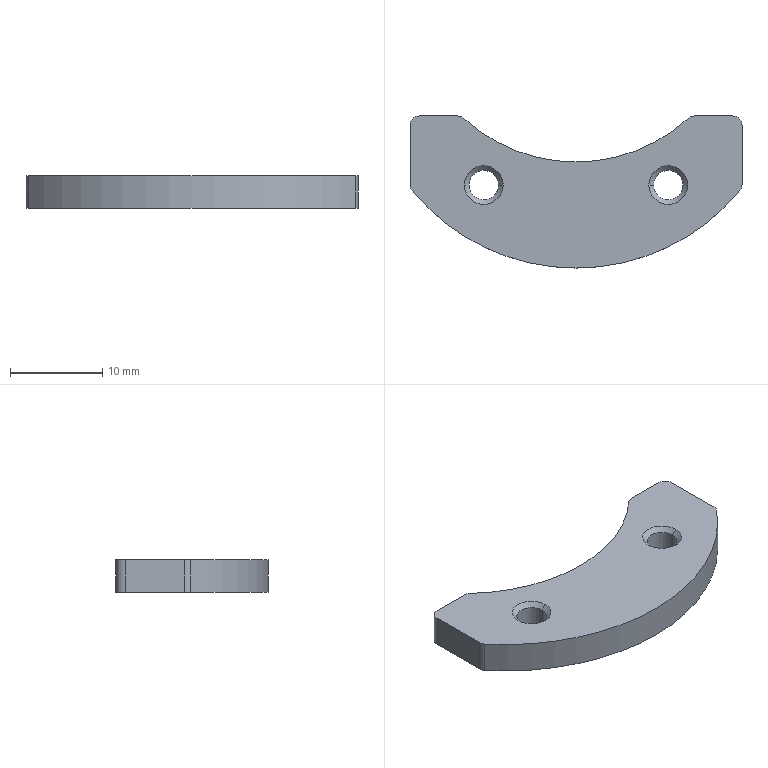Part | SolidWorks | features BaseBody 1 | 1 solid | 26 faces | box 36 x 16.5 x 3.5 mm | volume 1384 mm3 | cylinder 12 | cone 8 | plane 6 | commonest cylinder face diameters 2 x6 3.2 x4 36 x1 46 x1
STEP:
#1=CARTESIAN_POINT('',(-11.6,-20.5,3.));
#2=VERTEX_POINT('',#1);
#3=CARTESIAN_POINT('',(-8.4,-20.5,3.));
#4=VERTEX_POINT('',#3);
#5=CARTESIAN_POINT('',(-10.,-20.5,3.));
#6=DIRECTION('',(0.,0.,1.));
#7=DIRECTION('',(-1.,0.,0.));
#8=AXIS2_PLACEMENT_3D('',#5,#6,#7);
#9=CIRCLE('',#8,1.6);
#10=EDGE_CURVE('',#2,#4,#9,.T.);
#11=ORIENTED_EDGE('',*,*,#10,.F.);
#12=CARTESIAN_POINT('',(-12.1,-20.5,3.5));
#13=VERTEX_POINT('',#12);
#14=CARTESIAN_POINT('',(-11.6,-20.5,3.));
#15=DIRECTION('',(-0.7071,0.,0.7071));
#16=VECTOR('',#15,1000.);
#17=LINE('',#14,#16);
#18=EDGE_CURVE('',#2,#13,#17,.T.);
#19=ORIENTED_EDGE('',*,*,#18,.T.);
#20=CARTESIAN_POINT('',(-7.9,-20.5,3.5));
#21=VERTEX_POINT('',#20);
#22=CARTESIAN_POINT('',(-10.,-20.5,3.5));
#23=DIRECTION('',(0.,0.,-1.));
#24=DIRECTION('',(-1.,0.,0.));
#25=AXIS2_PLACEMENT_3D('',#22,#23,#24);
#26=CIRCLE('',#25,2.1);
#27=EDGE_CURVE('',#21,#13,#26,.T.);
#28=ORIENTED_EDGE('',*,*,#27,.F.);
#29=CARTESIAN_POINT('',(-8.4,-20.5,3.));
#30=DIRECTION('',(0.7071,0.,0.7071));
#31=VECTOR('',#30,1000.);
#32=LINE('',#29,#31);
#33=EDGE_CURVE('',#4,#21,#32,.T.);
#34=ORIENTED_EDGE('',*,*,#33,.F.);
#35=EDGE_LOOP('',(#11,#19,#28,#34));
#36=FACE_OUTER_BOUND('',#35,.T.);
#37=CARTESIAN_POINT('',(-10.,-20.5,3.));
#38=DIRECTION('',(0.,0.,1.));
#39=DIRECTION('',(1.,0.,0.));
#40=AXIS2_PLACEMENT_3D('',#37,#38,#39);
#41=CONICAL_SURFACE('',#40,1.6,0.7854);
#42=ADVANCED_FACE('',(#36),#41,.F.);
#43=CARTESIAN_POINT('',(-8.4,-20.5,0.5));
#44=VERTEX_POINT('',#43);
#45=CARTESIAN_POINT('',(-11.6,-20.5,0.5));
#46=VERTEX_POINT('',#45);
#47=CARTESIAN_POINT('',(-10.,-20.5,0.5));
#48=DIRECTION('',(0.,0.,-1.));
#49=DIRECTION('',(-1.,0.,0.));
#50=AXIS2_PLACEMENT_3D('',#47,#48,#49);
#51=CIRCLE('',#50,1.6);
#52=EDGE_CURVE('',#44,#46,#51,.T.);
#53=ORIENTED_EDGE('',*,*,#52,.F.);
#54=CARTESIAN_POINT('',(-7.9,-20.5,0.));
#55=VERTEX_POINT('',#54);
#56=CARTESIAN_POINT('',(-7.9,-20.5,0.));
#57=DIRECTION('',(0.7071,0.,-0.7071));
#58=VECTOR('',#57,1000.);
#59=LINE('',#56,#58);
#60=EDGE_CURVE('',#44,#55,#59,.T.);
#61=ORIENTED_EDGE('',*,*,#60,.T.);
#62=CARTESIAN_POINT('',(-12.1,-20.5,0.));
#63=VERTEX_POINT('',#62);
#64=CARTESIAN_POINT('',(-10.,-20.5,0.));
#65=DIRECTION('',(0.,0.,1.));
#66=DIRECTION('',(-1.,0.,0.));
#67=AXIS2_PLACEMENT_3D('',#64,#65,#66);
#68=CIRCLE('',#67,2.1);
#69=EDGE_CURVE('',#63,#55,#68,.T.);
#70=ORIENTED_EDGE('',*,*,#69,.F.);
#71=CARTESIAN_POINT('',(-12.1,-20.5,0.));
#72=DIRECTION('',(-0.7071,0.,-0.7071));
#73=VECTOR('',#72,1000.);
#74=LINE('',#71,#73);
#75=EDGE_CURVE('',#46,#63,#74,.T.);
#76=ORIENTED_EDGE('',*,*,#75,.F.);
#77=EDGE_LOOP('',(#53,#61,#70,#76));
#78=FACE_OUTER_BOUND('',#77,.T.);
#79=CARTESIAN_POINT('',(-10.,-20.5,0.));
#80=DIRECTION('',(0.,0.,-1.));
#81=DIRECTION('',(-1.,0.,0.));
#82=AXIS2_PLACEMENT_3D('',#79,#80,#81);
#83=CONICAL_SURFACE('',#82,2.1,0.7854);
#84=ADVANCED_FACE('',(#78),#83,.F.);
#85=CARTESIAN_POINT('',(8.4,-20.5,3.));
#86=VERTEX_POINT('',#85);
#87=CARTESIAN_POINT('',(11.6,-20.5,3.));
#88=VERTEX_POINT('',#87);
#89=CARTESIAN_POINT('',(10.,-20.5,3.));
#90=DIRECTION('',(0.,0.,1.));
#91=DIRECTION('',(-1.,0.,0.));
#92=AXIS2_PLACEMENT_3D('',#89,#90,#91);
#93=CIRCLE('',#92,1.6);
#94=EDGE_CURVE('',#86,#88,#93,.T.);
#95=ORIENTED_EDGE('',*,*,#94,.F.);
#96=CARTESIAN_POINT('',(7.9,-20.5,3.5));
#97=VERTEX_POINT('',#96);
#98=CARTESIAN_POINT('',(8.4,-20.5,3.));
#99=DIRECTION('',(-0.7071,0.,0.7071));
#100=VECTOR('',#99,1000.);
#101=LINE('',#98,#100);
#102=EDGE_CURVE('',#86,#97,#101,.T.);
#103=ORIENTED_EDGE('',*,*,#102,.T.);
#104=CARTESIAN_POINT('',(12.1,-20.5,3.5));
#105=VERTEX_POINT('',#104);
#106=CARTESIAN_POINT('',(10.,-20.5,3.5));
#107=DIRECTION('',(0.,0.,-1.));
#108=DIRECTION('',(-1.,0.,0.));
#109=AXIS2_PLACEMENT_3D('',#106,#107,#108);
#110=CIRCLE('',#109,2.1);
#111=EDGE_CURVE('',#105,#97,#110,.T.);
#112=ORIENTED_EDGE('',*,*,#111,.F.);
#113=CARTESIAN_POINT('',(11.6,-20.5,3.));
#114=DIRECTION('',(0.7071,0.,0.7071));
#115=VECTOR('',#114,1000.);
#116=LINE('',#113,#115);
#117=EDGE_CURVE('',#88,#105,#116,.T.);
#118=ORIENTED_EDGE('',*,*,#117,.F.);
#119=EDGE_LOOP('',(#95,#103,#112,#118));
#120=FACE_OUTER_BOUND('',#119,.T.);
#121=CARTESIAN_POINT('',(10.,-20.5,3.));
#122=DIRECTION('',(0.,0.,1.));
#123=DIRECTION('',(1.,0.,0.));
#124=AXIS2_PLACEMENT_3D('',#121,#122,#123);
#125=CONICAL_SURFACE('',#124,1.6,0.7854);
#126=ADVANCED_FACE('',(#120),#125,.F.);
#127=CARTESIAN_POINT('',(11.6,-20.5,0.5));
#128=VERTEX_POINT('',#127);
#129=CARTESIAN_POINT('',(8.4,-20.5,0.5));
#130=VERTEX_POINT('',#129);
#131=CARTESIAN_POINT('',(10.,-20.5,0.5));
#132=DIRECTION('',(0.,0.,-1.));
#133=DIRECTION('',(-1.,0.,0.));
#134=AXIS2_PLACEMENT_3D('',#131,#132,#133);
#135=CIRCLE('',#134,1.6);
#136=EDGE_CURVE('',#128,#130,#135,.T.);
#137=ORIENTED_EDGE('',*,*,#136,.F.);
#138=CARTESIAN_POINT('',(12.1,-20.5,0.));
#139=VERTEX_POINT('',#138);
#140=CARTESIAN_POINT('',(12.1,-20.5,0.));
#141=DIRECTION('',(0.7071,0.,-0.7071));
#142=VECTOR('',#141,1000.);
#143=LINE('',#140,#142);
#144=EDGE_CURVE('',#128,#139,#143,.T.);
#145=ORIENTED_EDGE('',*,*,#144,.T.);
#146=CARTESIAN_POINT('',(7.9,-20.5,0.));
#147=VERTEX_POINT('',#146);
#148=CARTESIAN_POINT('',(10.,-20.5,0.));
#149=DIRECTION('',(0.,0.,1.));
#150=DIRECTION('',(-1.,0.,0.));
#151=AXIS2_PLACEMENT_3D('',#148,#149,#150);
#152=CIRCLE('',#151,2.1);
#153=EDGE_CURVE('',#147,#139,#152,.T.);
#154=ORIENTED_EDGE('',*,*,#153,.F.);
#155=CARTESIAN_POINT('',(7.9,-20.5,0.));
#156=DIRECTION('',(-0.7071,0.,-0.7071));
#157=VECTOR('',#156,1000.);
#158=LINE('',#155,#157);
#159=EDGE_CURVE('',#130,#147,#158,.T.);
#160=ORIENTED_EDGE('',*,*,#159,.F.);
#161=EDGE_LOOP('',(#137,#145,#154,#160));
#162=FACE_OUTER_BOUND('',#161,.T.);
#163=CARTESIAN_POINT('',(10.,-20.5,0.));
#164=DIRECTION('',(0.,0.,-1.));
#165=DIRECTION('',(-1.,0.,0.));
#166=AXIS2_PLACEMENT_3D('',#163,#164,#165);
#167=CONICAL_SURFACE('',#166,2.1,0.7854);
#168=ADVANCED_FACE('',(#162),#167,.F.);
#169=ORIENTED_EDGE('',*,*,#94,.T.);
#170=CARTESIAN_POINT('',(11.6,-20.5,3.5));
#171=DIRECTION('',(0.,0.,-1.));
#172=VECTOR('',#171,1000.);
#173=LINE('',#170,#172);
#174=EDGE_CURVE('',#88,#128,#173,.T.);
#175=ORIENTED_EDGE('',*,*,#174,.T.);
#176=ORIENTED_EDGE('',*,*,#136,.T.);
#177=CARTESIAN_POINT('',(8.4,-20.5,3.5));
#178=DIRECTION('',(0.,0.,-1.));
#179=VECTOR('',#178,1000.);
#180=LINE('',#177,#179);
#181=EDGE_CURVE('',#86,#130,#180,.T.);
#182=ORIENTED_EDGE('',*,*,#181,.F.);
#183=EDGE_LOOP('',(#169,#175,#176,#182));
#184=FACE_OUTER_BOUND('',#183,.T.);
#185=CARTESIAN_POINT('',(10.,-20.5,3.5));
#186=DIRECTION('',(0.,0.,-1.));
#187=DIRECTION('',(-1.,0.,0.));
#188=AXIS2_PLACEMENT_3D('',#185,#186,#187);
#189=CYLINDRICAL_SURFACE('',#188,1.6);
#190=ADVANCED_FACE('',(#184),#189,.F.);
#191=ORIENTED_EDGE('',*,*,#10,.T.);
#192=CARTESIAN_POINT('',(-8.4,-20.5,3.5));
#193=DIRECTION('',(0.,0.,-1.));
#194=VECTOR('',#193,1000.);
#195=LINE('',#192,#194);
#196=EDGE_CURVE('',#4,#44,#195,.T.);
#197=ORIENTED_EDGE('',*,*,#196,.T.);
#198=ORIENTED_EDGE('',*,*,#52,.T.);
#199=CARTESIAN_POINT('',(-11.6,-20.5,3.5));
#200=DIRECTION('',(0.,0.,-1.));
#201=VECTOR('',#200,1000.);
#202=LINE('',#199,#201);
#203=EDGE_CURVE('',#2,#46,#202,.T.);
#204=ORIENTED_EDGE('',*,*,#203,.F.);
#205=EDGE_LOOP('',(#191,#197,#198,#204));
#206=FACE_OUTER_BOUND('',#205,.T.);
#207=CARTESIAN_POINT('',(-10.,-20.5,3.5));
#208=DIRECTION('',(0.,0.,-1.));
#209=DIRECTION('',(-1.,0.,0.));
#210=AXIS2_PLACEMENT_3D('',#207,#208,#209);
#211=CYLINDRICAL_SURFACE('',#210,1.6);
#212=ADVANCED_FACE('',(#206),#211,.F.);
#213=ORIENTED_EDGE('',*,*,#111,.T.);
#214=CARTESIAN_POINT('',(10.,-20.5,3.5));
#215=DIRECTION('',(0.,0.,-1.));
#216=DIRECTION('',(-1.,0.,0.));
#217=AXIS2_PLACEMENT_3D('',#214,#215,#216);
#218=CIRCLE('',#217,2.1);
#219=EDGE_CURVE('',#97,#105,#218,.T.);
#220=ORIENTED_EDGE('',*,*,#219,.T.);
#221=EDGE_LOOP('',(#213,#220));
#222=FACE_BOUND('',#221,.T.);
#223=ORIENTED_EDGE('',*,*,#27,.T.);
#224=CARTESIAN_POINT('',(-10.,-20.5,3.5));
#225=DIRECTION('',(0.,0.,-1.));
#226=DIRECTION('',(-1.,0.,0.));
#227=AXIS2_PLACEMENT_3D('',#224,#225,#226);
#228=CIRCLE('',#227,2.1);
#229=EDGE_CURVE('',#13,#21,#228,.T.);
#230=ORIENTED_EDGE('',*,*,#229,.T.);
#231=EDGE_LOOP('',(#223,#230));
#232=FACE_BOUND('',#231,.T.);
#233=CARTESIAN_POINT('',(-18.,-20.464,3.5));
#234=VERTEX_POINT('',#233);
#235=CARTESIAN_POINT('',(-17.773,-21.099,3.5));
#236=VERTEX_POINT('',#235);
#237=CARTESIAN_POINT('',(-17.,-20.464,3.5));
#238=DIRECTION('',(0.,0.,1.));
#239=DIRECTION('',(-1.,0.,0.));
#240=AXIS2_PLACEMENT_3D('',#237,#238,#239);
#241=CIRCLE('',#240,1.);
#242=EDGE_CURVE('',#234,#236,#241,.T.);
#243=ORIENTED_EDGE('',*,*,#242,.T.);
#244=CARTESIAN_POINT('',(17.773,-21.099,3.5));
#245=VERTEX_POINT('',#244);
#246=CARTESIAN_POINT('',(0.,-6.5,3.5));
#247=DIRECTION('',(0.,0.,1.));
#248=DIRECTION('',(1.,0.,0.));
#249=AXIS2_PLACEMENT_3D('',#246,#247,#248);
#250=CIRCLE('',#249,23.);
#251=EDGE_CURVE('',#236,#245,#250,.T.);
#252=ORIENTED_EDGE('',*,*,#251,.T.);
#253=CARTESIAN_POINT('',(18.,-20.464,3.5));
#254=VERTEX_POINT('',#253);
#255=CARTESIAN_POINT('',(17.,-20.464,3.5));
#256=DIRECTION('',(0.,0.,1.));
#257=DIRECTION('',(-1.,0.,0.));
#258=AXIS2_PLACEMENT_3D('',#255,#256,#257);
#259=CIRCLE('',#258,1.);
#260=EDGE_CURVE('',#245,#254,#259,.T.);
#261=ORIENTED_EDGE('',*,*,#260,.T.);
#262=CARTESIAN_POINT('',(18.,-14.,3.5));
#263=VERTEX_POINT('',#262);
#264=CARTESIAN_POINT('',(18.,-20.464,3.5));
#265=DIRECTION('',(0.,1.,0.));
#266=VECTOR('',#265,1000.);
#267=LINE('',#264,#266);
#268=EDGE_CURVE('',#254,#263,#267,.T.);
#269=ORIENTED_EDGE('',*,*,#268,.T.);
#270=CARTESIAN_POINT('',(17.,-13.,3.5));
#271=VERTEX_POINT('',#270);
#272=CARTESIAN_POINT('',(17.,-14.,3.5));
#273=DIRECTION('',(0.,0.,1.));
#274=DIRECTION('',(1.,0.,0.));
#275=AXIS2_PLACEMENT_3D('',#272,#273,#274);
#276=CIRCLE('',#275,1.);
#277=EDGE_CURVE('',#263,#271,#276,.T.);
#278=ORIENTED_EDGE('',*,*,#277,.T.);
#279=CARTESIAN_POINT('',(12.845,-13.,3.5));
#280=VERTEX_POINT('',#279);
#281=CARTESIAN_POINT('',(12.845,-13.,3.5));
#282=DIRECTION('',(-1.,0.,0.));
#283=VECTOR('',#282,1000.);
#284=LINE('',#281,#283);
#285=EDGE_CURVE('',#271,#280,#284,.T.);
#286=ORIENTED_EDGE('',*,*,#285,.T.);
#287=CARTESIAN_POINT('',(12.169,-13.263,3.5));
#288=VERTEX_POINT('',#287);
#289=CARTESIAN_POINT('',(12.845,-14.,3.5));
#290=DIRECTION('',(0.,0.,1.));
#291=DIRECTION('',(1.,0.,0.));
#292=AXIS2_PLACEMENT_3D('',#289,#290,#291);
#293=CIRCLE('',#292,1.);
#294=EDGE_CURVE('',#280,#288,#293,.T.);
#295=ORIENTED_EDGE('',*,*,#294,.T.);
#296=CARTESIAN_POINT('',(-12.169,-13.263,3.5));
#297=VERTEX_POINT('',#296);
#298=CARTESIAN_POINT('',(0.,0.,3.5));
#299=DIRECTION('',(0.,0.,-1.));
#300=DIRECTION('',(1.,0.,0.));
#301=AXIS2_PLACEMENT_3D('',#298,#299,#300);
#302=CIRCLE('',#301,18.);
#303=EDGE_CURVE('',#288,#297,#302,.T.);
#304=ORIENTED_EDGE('',*,*,#303,.T.);
#305=CARTESIAN_POINT('',(-12.845,-13.,3.5));
#306=VERTEX_POINT('',#305);
#307=CARTESIAN_POINT('',(-12.845,-14.,3.5));
#308=DIRECTION('',(0.,0.,1.));
#309=DIRECTION('',(1.,0.,0.));
#310=AXIS2_PLACEMENT_3D('',#307,#308,#309);
#311=CIRCLE('',#310,1.);
#312=EDGE_CURVE('',#297,#306,#311,.T.);
#313=ORIENTED_EDGE('',*,*,#312,.T.);
#314=CARTESIAN_POINT('',(-17.,-13.,3.5));
#315=VERTEX_POINT('',#314);
#316=CARTESIAN_POINT('',(-17.,-13.,3.5));
#317=DIRECTION('',(-1.,0.,0.));
#318=VECTOR('',#317,1000.);
#319=LINE('',#316,#318);
#320=EDGE_CURVE('',#306,#315,#319,.T.);
#321=ORIENTED_EDGE('',*,*,#320,.T.);
#322=CARTESIAN_POINT('',(-18.,-14.,3.5));
#323=VERTEX_POINT('',#322);
#324=CARTESIAN_POINT('',(-17.,-14.,3.5));
#325=DIRECTION('',(0.,0.,1.));
#326=DIRECTION('',(1.,0.,0.));
#327=AXIS2_PLACEMENT_3D('',#324,#325,#326);
#328=CIRCLE('',#327,1.);
#329=EDGE_CURVE('',#315,#323,#328,.T.);
#330=ORIENTED_EDGE('',*,*,#329,.T.);
#331=CARTESIAN_POINT('',(-18.,-20.464,3.5));
#332=DIRECTION('',(0.,-1.,0.));
#333=VECTOR('',#332,1000.);
#334=LINE('',#331,#333);
#335=EDGE_CURVE('',#323,#234,#334,.T.);
#336=ORIENTED_EDGE('',*,*,#335,.T.);
#337=EDGE_LOOP('',(#243,#252,#261,#269,#278,#286,#295,#304,#313,#321,#330,#336));
#338=FACE_OUTER_BOUND('',#337,.T.);
#339=CARTESIAN_POINT('',(-17.,-20.464,3.5));
#340=DIRECTION('',(0.,0.,-1.));
#341=DIRECTION('',(-1.,0.,0.));
#342=AXIS2_PLACEMENT_3D('',#339,#340,#341);
#343=PLANE('',#342);
#344=ADVANCED_FACE('',(#222,#232,#338),#343,.F.);
#345=ORIENTED_EDGE('',*,*,#153,.T.);
#346=CARTESIAN_POINT('',(10.,-20.5,0.));
#347=DIRECTION('',(0.,0.,1.));
#348=DIRECTION('',(-1.,0.,0.));
#349=AXIS2_PLACEMENT_3D('',#346,#347,#348);
#350=CIRCLE('',#349,2.1);
#351=EDGE_CURVE('',#139,#147,#350,.T.);
#352=ORIENTED_EDGE('',*,*,#351,.T.);
#353=EDGE_LOOP('',(#345,#352));
#354=FACE_BOUND('',#353,.T.);
#355=ORIENTED_EDGE('',*,*,#69,.T.);
#356=CARTESIAN_POINT('',(-10.,-20.5,0.));
#357=DIRECTION('',(0.,0.,1.));
#358=DIRECTION('',(-1.,0.,0.));
#359=AXIS2_PLACEMENT_3D('',#356,#357,#358);
#360=CIRCLE('',#359,2.1);
#361=EDGE_CURVE('',#55,#63,#360,.T.);
#362=ORIENTED_EDGE('',*,*,#361,.T.);
#363=EDGE_LOOP('',(#355,#362));
#364=FACE_BOUND('',#363,.T.);
#365=CARTESIAN_POINT('',(-18.,-20.464,0.));
#366=VERTEX_POINT('',#365);
#367=CARTESIAN_POINT('',(-17.773,-21.099,0.));
#368=VERTEX_POINT('',#367);
#369=CARTESIAN_POINT('',(-17.,-20.464,0.));
#370=DIRECTION('',(0.,0.,1.));
#371=DIRECTION('',(-1.,0.,0.));
#372=AXIS2_PLACEMENT_3D('',#369,#370,#371);
#373=CIRCLE('',#372,1.);
#374=EDGE_CURVE('',#366,#368,#373,.T.);
#375=ORIENTED_EDGE('',*,*,#374,.F.);
#376=CARTESIAN_POINT('',(-18.,-14.,0.));
#377=VERTEX_POINT('',#376);
#378=CARTESIAN_POINT('',(-18.,-20.464,0.));
#379=DIRECTION('',(0.,-1.,0.));
#380=VECTOR('',#379,1000.);
#381=LINE('',#378,#380);
#382=EDGE_CURVE('',#377,#366,#381,.T.);
#383=ORIENTED_EDGE('',*,*,#382,.F.);
#384=CARTESIAN_POINT('',(-17.,-13.,0.));
#385=VERTEX_POINT('',#384);
#386=CARTESIAN_POINT('',(-17.,-14.,0.));
#387=DIRECTION('',(0.,0.,1.));
#388=DIRECTION('',(1.,0.,0.));
#389=AXIS2_PLACEMENT_3D('',#386,#387,#388);
#390=CIRCLE('',#389,1.);
#391=EDGE_CURVE('',#385,#377,#390,.T.);
#392=ORIENTED_EDGE('',*,*,#391,.F.);
#393=CARTESIAN_POINT('',(-12.845,-13.,0.));
#394=VERTEX_POINT('',#393);
#395=CARTESIAN_POINT('',(-17.,-13.,0.));
#396=DIRECTION('',(-1.,0.,0.));
#397=VECTOR('',#396,1000.);
#398=LINE('',#395,#397);
#399=EDGE_CURVE('',#394,#385,#398,.T.);
#400=ORIENTED_EDGE('',*,*,#399,.F.);
#401=CARTESIAN_POINT('',(-12.169,-13.263,0.));
#402=VERTEX_POINT('',#401);
#403=CARTESIAN_POINT('',(-12.845,-14.,0.));
#404=DIRECTION('',(0.,0.,1.));
#405=DIRECTION('',(1.,0.,0.));
#406=AXIS2_PLACEMENT_3D('',#403,#404,#405);
#407=CIRCLE('',#406,1.);
#408=EDGE_CURVE('',#402,#394,#407,.T.);
#409=ORIENTED_EDGE('',*,*,#408,.F.);
#410=CARTESIAN_POINT('',(12.169,-13.263,0.));
#411=VERTEX_POINT('',#410);
#412=CARTESIAN_POINT('',(0.,0.,0.));
#413=DIRECTION('',(0.,0.,-1.));
#414=DIRECTION('',(1.,0.,0.));
#415=AXIS2_PLACEMENT_3D('',#412,#413,#414);
#416=CIRCLE('',#415,18.);
#417=EDGE_CURVE('',#411,#402,#416,.T.);
#418=ORIENTED_EDGE('',*,*,#417,.F.);
#419=CARTESIAN_POINT('',(12.845,-13.,0.));
#420=VERTEX_POINT('',#419);
#421=CARTESIAN_POINT('',(12.845,-14.,0.));
#422=DIRECTION('',(0.,0.,1.));
#423=DIRECTION('',(1.,0.,0.));
#424=AXIS2_PLACEMENT_3D('',#421,#422,#423);
#425=CIRCLE('',#424,1.);
#426=EDGE_CURVE('',#420,#411,#425,.T.);
#427=ORIENTED_EDGE('',*,*,#426,.F.);
#428=CARTESIAN_POINT('',(17.,-13.,0.));
#429=VERTEX_POINT('',#428);
#430=CARTESIAN_POINT('',(12.845,-13.,0.));
#431=DIRECTION('',(-1.,0.,0.));
#432=VECTOR('',#431,1000.);
#433=LINE('',#430,#432);
#434=EDGE_CURVE('',#429,#420,#433,.T.);
#435=ORIENTED_EDGE('',*,*,#434,.F.);
#436=CARTESIAN_POINT('',(18.,-14.,0.));
#437=VERTEX_POINT('',#436);
#438=CARTESIAN_POINT('',(17.,-14.,0.));
#439=DIRECTION('',(0.,0.,1.));
#440=DIRECTION('',(1.,0.,0.));
#441=AXIS2_PLACEMENT_3D('',#438,#439,#440);
#442=CIRCLE('',#441,1.);
#443=EDGE_CURVE('',#437,#429,#442,.T.);
#444=ORIENTED_EDGE('',*,*,#443,.F.);
#445=CARTESIAN_POINT('',(18.,-20.464,0.));
#446=VERTEX_POINT('',#445);
#447=CARTESIAN_POINT('',(18.,-20.464,0.));
#448=DIRECTION('',(0.,1.,0.));
#449=VECTOR('',#448,1000.);
#450=LINE('',#447,#449);
#451=EDGE_CURVE('',#446,#437,#450,.T.);
#452=ORIENTED_EDGE('',*,*,#451,.F.);
#453=CARTESIAN_POINT('',(17.773,-21.099,0.));
#454=VERTEX_POINT('',#453);
#455=CARTESIAN_POINT('',(17.,-20.464,0.));
#456=DIRECTION('',(0.,0.,1.));
#457=DIRECTION('',(-1.,0.,0.));
#458=AXIS2_PLACEMENT_3D('',#455,#456,#457);
#459=CIRCLE('',#458,1.);
#460=EDGE_CURVE('',#454,#446,#459,.T.);
#461=ORIENTED_EDGE('',*,*,#460,.F.);
#462=CARTESIAN_POINT('',(0.,-6.5,0.));
#463=DIRECTION('',(0.,0.,1.));
#464=DIRECTION('',(1.,0.,0.));
#465=AXIS2_PLACEMENT_3D('',#462,#463,#464);
#466=CIRCLE('',#465,23.);
#467=EDGE_CURVE('',#368,#454,#466,.T.);
#468=ORIENTED_EDGE('',*,*,#467,.F.);
#469=EDGE_LOOP('',(#375,#383,#392,#400,#409,#418,#427,#435,#444,#452,#461,#468));
#470=FACE_OUTER_BOUND('',#469,.T.);
#471=CARTESIAN_POINT('',(-17.,-20.464,0.));
#472=DIRECTION('',(0.,0.,-1.));
#473=DIRECTION('',(-1.,0.,0.));
#474=AXIS2_PLACEMENT_3D('',#471,#472,#473);
#475=PLANE('',#474);
#476=ADVANCED_FACE('',(#354,#364,#470),#475,.T.);
#477=ORIENTED_EDGE('',*,*,#374,.T.);
#478=CARTESIAN_POINT('',(-17.773,-21.099,3.5));
#479=DIRECTION('',(0.,0.,-1.));
#480=VECTOR('',#479,1000.);
#481=LINE('',#478,#480);
#482=EDGE_CURVE('',#236,#368,#481,.T.);
#483=ORIENTED_EDGE('',*,*,#482,.F.);
#484=ORIENTED_EDGE('',*,*,#242,.F.);
#485=CARTESIAN_POINT('',(-18.,-20.464,3.5));
#486=DIRECTION('',(0.,0.,-1.));
#487=VECTOR('',#486,1000.);
#488=LINE('',#485,#487);
#489=EDGE_CURVE('',#234,#366,#488,.T.);
#490=ORIENTED_EDGE('',*,*,#489,.T.);
#491=EDGE_LOOP('',(#477,#483,#484,#490));
#492=FACE_OUTER_BOUND('',#491,.T.);
#493=CARTESIAN_POINT('',(-17.,-20.464,3.5));
#494=DIRECTION('',(0.,0.,-1.));
#495=DIRECTION('',(-1.,0.,0.));
#496=AXIS2_PLACEMENT_3D('',#493,#494,#495);
#497=CYLINDRICAL_SURFACE('',#496,1.);
#498=ADVANCED_FACE('',(#492),#497,.T.);
#499=ORIENTED_EDGE('',*,*,#467,.T.);
#500=CARTESIAN_POINT('',(17.773,-21.099,3.5));
#501=DIRECTION('',(0.,0.,-1.));
#502=VECTOR('',#501,1000.);
#503=LINE('',#500,#502);
#504=EDGE_CURVE('',#245,#454,#503,.T.);
#505=ORIENTED_EDGE('',*,*,#504,.F.);
#506=ORIENTED_EDGE('',*,*,#251,.F.);
#507=ORIENTED_EDGE('',*,*,#482,.T.);
#508=EDGE_LOOP('',(#499,#505,#506,#507));
#509=FACE_OUTER_BOUND('',#508,.T.);
#510=CARTESIAN_POINT('',(0.,-6.5,3.5));
#511=DIRECTION('',(0.,0.,-1.));
#512=DIRECTION('',(-1.,0.,0.));
#513=AXIS2_PLACEMENT_3D('',#510,#511,#512);
#514=CYLINDRICAL_SURFACE('',#513,23.);
#515=ADVANCED_FACE('',(#509),#514,.T.);
#516=ORIENTED_EDGE('',*,*,#460,.T.);
#517=CARTESIAN_POINT('',(18.,-20.464,3.5));
#518=DIRECTION('',(0.,0.,-1.));
#519=VECTOR('',#518,1000.);
#520=LINE('',#517,#519);
#521=EDGE_CURVE('',#254,#446,#520,.T.);
#522=ORIENTED_EDGE('',*,*,#521,.F.);
#523=ORIENTED_EDGE('',*,*,#260,.F.);
#524=ORIENTED_EDGE('',*,*,#504,.T.);
#525=EDGE_LOOP('',(#516,#522,#523,#524));
#526=FACE_OUTER_BOUND('',#525,.T.);
#527=CARTESIAN_POINT('',(17.,-20.464,3.5));
#528=DIRECTION('',(0.,0.,-1.));
#529=DIRECTION('',(-1.,0.,0.));
#530=AXIS2_PLACEMENT_3D('',#527,#528,#529);
#531=CYLINDRICAL_SURFACE('',#530,1.);
#532=ADVANCED_FACE('',(#526),#531,.T.);
#533=ORIENTED_EDGE('',*,*,#451,.T.);
#534=CARTESIAN_POINT('',(18.,-14.,3.5));
#535=DIRECTION('',(0.,0.,-1.));
#536=VECTOR('',#535,1000.);
#537=LINE('',#534,#536);
#538=EDGE_CURVE('',#263,#437,#537,.T.);
#539=ORIENTED_EDGE('',*,*,#538,.F.);
#540=ORIENTED_EDGE('',*,*,#268,.F.);
#541=ORIENTED_EDGE('',*,*,#521,.T.);
#542=EDGE_LOOP('',(#533,#539,#540,#541));
#543=FACE_OUTER_BOUND('',#542,.T.);
#544=CARTESIAN_POINT('',(18.,-20.464,3.5));
#545=DIRECTION('',(-1.,0.,0.));
#546=DIRECTION('',(0.,0.,1.));
#547=AXIS2_PLACEMENT_3D('',#544,#545,#546);
#548=PLANE('',#547);
#549=ADVANCED_FACE('',(#543),#548,.F.);
#550=ORIENTED_EDGE('',*,*,#443,.T.);
#551=CARTESIAN_POINT('',(17.,-13.,3.5));
#552=DIRECTION('',(0.,0.,-1.));
#553=VECTOR('',#552,1000.);
#554=LINE('',#551,#553);
#555=EDGE_CURVE('',#271,#429,#554,.T.);
#556=ORIENTED_EDGE('',*,*,#555,.F.);
#557=ORIENTED_EDGE('',*,*,#277,.F.);
#558=ORIENTED_EDGE('',*,*,#538,.T.);
#559=EDGE_LOOP('',(#550,#556,#557,#558));
#560=FACE_OUTER_BOUND('',#559,.T.);
#561=CARTESIAN_POINT('',(17.,-14.,3.5));
#562=DIRECTION('',(0.,0.,-1.));
#563=DIRECTION('',(-1.,0.,0.));
#564=AXIS2_PLACEMENT_3D('',#561,#562,#563);
#565=CYLINDRICAL_SURFACE('',#564,1.);
#566=ADVANCED_FACE('',(#560),#565,.T.);
#567=ORIENTED_EDGE('',*,*,#434,.T.);
#568=CARTESIAN_POINT('',(12.845,-13.,3.5));
#569=DIRECTION('',(0.,0.,-1.));
#570=VECTOR('',#569,1000.);
#571=LINE('',#568,#570);
#572=EDGE_CURVE('',#280,#420,#571,.T.);
#573=ORIENTED_EDGE('',*,*,#572,.F.);
#574=ORIENTED_EDGE('',*,*,#285,.F.);
#575=ORIENTED_EDGE('',*,*,#555,.T.);
#576=EDGE_LOOP('',(#567,#573,#574,#575));
#577=FACE_OUTER_BOUND('',#576,.T.);
#578=CARTESIAN_POINT('',(12.845,-13.,3.5));
#579=DIRECTION('',(0.,-1.,0.));
#580=DIRECTION('',(0.,0.,-1.));
#581=AXIS2_PLACEMENT_3D('',#578,#579,#580);
#582=PLANE('',#581);
#583=ADVANCED_FACE('',(#577),#582,.F.);
#584=ORIENTED_EDGE('',*,*,#426,.T.);
#585=CARTESIAN_POINT('',(12.169,-13.263,3.5));
#586=DIRECTION('',(0.,0.,-1.));
#587=VECTOR('',#586,1000.);
#588=LINE('',#585,#587);
#589=EDGE_CURVE('',#288,#411,#588,.T.);
#590=ORIENTED_EDGE('',*,*,#589,.F.);
#591=ORIENTED_EDGE('',*,*,#294,.F.);
#592=ORIENTED_EDGE('',*,*,#572,.T.);
#593=EDGE_LOOP('',(#584,#590,#591,#592));
#594=FACE_OUTER_BOUND('',#593,.T.);
#595=CARTESIAN_POINT('',(12.845,-14.,3.5));
#596=DIRECTION('',(0.,0.,-1.));
#597=DIRECTION('',(-1.,0.,0.));
#598=AXIS2_PLACEMENT_3D('',#595,#596,#597);
#599=CYLINDRICAL_SURFACE('',#598,1.);
#600=ADVANCED_FACE('',(#594),#599,.T.);
#601=ORIENTED_EDGE('',*,*,#417,.T.);
#602=CARTESIAN_POINT('',(-12.169,-13.263,3.5));
#603=DIRECTION('',(0.,0.,-1.));
#604=VECTOR('',#603,1000.);
#605=LINE('',#602,#604);
#606=EDGE_CURVE('',#297,#402,#605,.T.);
#607=ORIENTED_EDGE('',*,*,#606,.F.);
#608=ORIENTED_EDGE('',*,*,#303,.F.);
#609=ORIENTED_EDGE('',*,*,#589,.T.);
#610=EDGE_LOOP('',(#601,#607,#608,#609));
#611=FACE_OUTER_BOUND('',#610,.T.);
#612=CARTESIAN_POINT('',(0.,0.,3.5));
#613=DIRECTION('',(0.,0.,-1.));
#614=DIRECTION('',(-1.,0.,0.));
#615=AXIS2_PLACEMENT_3D('',#612,#613,#614);
#616=CYLINDRICAL_SURFACE('',#615,18.);
#617=ADVANCED_FACE('',(#611),#616,.F.);
#618=ORIENTED_EDGE('',*,*,#408,.T.);
#619=CARTESIAN_POINT('',(-12.845,-13.,3.5));
#620=DIRECTION('',(0.,0.,-1.));
#621=VECTOR('',#620,1000.);
#622=LINE('',#619,#621);
#623=EDGE_CURVE('',#306,#394,#622,.T.);
#624=ORIENTED_EDGE('',*,*,#623,.F.);
#625=ORIENTED_EDGE('',*,*,#312,.F.);
#626=ORIENTED_EDGE('',*,*,#606,.T.);
#627=EDGE_LOOP('',(#618,#624,#625,#626));
#628=FACE_OUTER_BOUND('',#627,.T.);
#629=CARTESIAN_POINT('',(-12.845,-14.,3.5));
#630=DIRECTION('',(0.,0.,-1.));
#631=DIRECTION('',(-1.,0.,0.));
#632=AXIS2_PLACEMENT_3D('',#629,#630,#631);
#633=CYLINDRICAL_SURFACE('',#632,1.);
#634=ADVANCED_FACE('',(#628),#633,.T.);
#635=ORIENTED_EDGE('',*,*,#399,.T.);
#636=CARTESIAN_POINT('',(-17.,-13.,3.5));
#637=DIRECTION('',(0.,0.,-1.));
#638=VECTOR('',#637,1000.);
#639=LINE('',#636,#638);
#640=EDGE_CURVE('',#315,#385,#639,.T.);
#641=ORIENTED_EDGE('',*,*,#640,.F.);
#642=ORIENTED_EDGE('',*,*,#320,.F.);
#643=ORIENTED_EDGE('',*,*,#623,.T.);
#644=EDGE_LOOP('',(#635,#641,#642,#643));
#645=FACE_OUTER_BOUND('',#644,.T.);
#646=CARTESIAN_POINT('',(-17.,-13.,3.5));
#647=DIRECTION('',(0.,-1.,0.));
#648=DIRECTION('',(0.,0.,-1.));
#649=AXIS2_PLACEMENT_3D('',#646,#647,#648);
#650=PLANE('',#649);
#651=ADVANCED_FACE('',(#645),#650,.F.);
#652=ORIENTED_EDGE('',*,*,#391,.T.);
#653=CARTESIAN_POINT('',(-18.,-14.,3.5));
#654=DIRECTION('',(0.,0.,-1.));
#655=VECTOR('',#654,1000.);
#656=LINE('',#653,#655);
#657=EDGE_CURVE('',#323,#377,#656,.T.);
#658=ORIENTED_EDGE('',*,*,#657,.F.);
#659=ORIENTED_EDGE('',*,*,#329,.F.);
#660=ORIENTED_EDGE('',*,*,#640,.T.);
#661=EDGE_LOOP('',(#652,#658,#659,#660));
#662=FACE_OUTER_BOUND('',#661,.T.);
#663=CARTESIAN_POINT('',(-17.,-14.,3.5));
#664=DIRECTION('',(0.,0.,-1.));
#665=DIRECTION('',(-1.,0.,0.));
#666=AXIS2_PLACEMENT_3D('',#663,#664,#665);
#667=CYLINDRICAL_SURFACE('',#666,1.);
#668=ADVANCED_FACE('',(#662),#667,.T.);
#669=ORIENTED_EDGE('',*,*,#382,.T.);
#670=ORIENTED_EDGE('',*,*,#489,.F.);
#671=ORIENTED_EDGE('',*,*,#335,.F.);
#672=ORIENTED_EDGE('',*,*,#657,.T.);
#673=EDGE_LOOP('',(#669,#670,#671,#672));
#674=FACE_OUTER_BOUND('',#673,.T.);
#675=CARTESIAN_POINT('',(-18.,-20.464,3.5));
#676=DIRECTION('',(1.,0.,0.));
#677=DIRECTION('',(0.,0.,-1.));
#678=AXIS2_PLACEMENT_3D('',#675,#676,#677);
#679=PLANE('',#678);
#680=ADVANCED_FACE('',(#674),#679,.F.);
#681=ORIENTED_EDGE('',*,*,#196,.F.);
#682=CARTESIAN_POINT('',(-10.,-20.5,3.));
#683=DIRECTION('',(0.,0.,1.));
#684=DIRECTION('',(-1.,0.,0.));
#685=AXIS2_PLACEMENT_3D('',#682,#683,#684);
#686=CIRCLE('',#685,1.6);
#687=EDGE_CURVE('',#4,#2,#686,.T.);
#688=ORIENTED_EDGE('',*,*,#687,.T.);
#689=ORIENTED_EDGE('',*,*,#203,.T.);
#690=CARTESIAN_POINT('',(-10.,-20.5,0.5));
#691=DIRECTION('',(0.,0.,-1.));
#692=DIRECTION('',(-1.,0.,0.));
#693=AXIS2_PLACEMENT_3D('',#690,#691,#692);
#694=CIRCLE('',#693,1.6);
#695=EDGE_CURVE('',#46,#44,#694,.T.);
#696=ORIENTED_EDGE('',*,*,#695,.T.);
#697=EDGE_LOOP('',(#681,#688,#689,#696));
#698=FACE_OUTER_BOUND('',#697,.T.);
#699=CARTESIAN_POINT('',(-10.,-20.5,3.5));
#700=DIRECTION('',(0.,0.,-1.));
#701=DIRECTION('',(-1.,0.,0.));
#702=AXIS2_PLACEMENT_3D('',#699,#700,#701);
#703=CYLINDRICAL_SURFACE('',#702,1.6);
#704=ADVANCED_FACE('',(#698),#703,.F.);
#705=ORIENTED_EDGE('',*,*,#174,.F.);
#706=CARTESIAN_POINT('',(10.,-20.5,3.));
#707=DIRECTION('',(0.,0.,1.));
#708=DIRECTION('',(-1.,0.,0.));
#709=AXIS2_PLACEMENT_3D('',#706,#707,#708);
#710=CIRCLE('',#709,1.6);
#711=EDGE_CURVE('',#88,#86,#710,.T.);
#712=ORIENTED_EDGE('',*,*,#711,.T.);
#713=ORIENTED_EDGE('',*,*,#181,.T.);
#714=CARTESIAN_POINT('',(10.,-20.5,0.5));
#715=DIRECTION('',(0.,0.,-1.));
#716=DIRECTION('',(-1.,0.,0.));
#717=AXIS2_PLACEMENT_3D('',#714,#715,#716);
#718=CIRCLE('',#717,1.6);
#719=EDGE_CURVE('',#130,#128,#718,.T.);
#720=ORIENTED_EDGE('',*,*,#719,.T.);
#721=EDGE_LOOP('',(#705,#712,#713,#720));
#722=FACE_OUTER_BOUND('',#721,.T.);
#723=CARTESIAN_POINT('',(10.,-20.5,3.5));
#724=DIRECTION('',(0.,0.,-1.));
#725=DIRECTION('',(-1.,0.,0.));
#726=AXIS2_PLACEMENT_3D('',#723,#724,#725);
#727=CYLINDRICAL_SURFACE('',#726,1.6);
#728=ADVANCED_FACE('',(#722),#727,.F.);
#729=ORIENTED_EDGE('',*,*,#144,.F.);
#730=ORIENTED_EDGE('',*,*,#719,.F.);
#731=ORIENTED_EDGE('',*,*,#159,.T.);
#732=ORIENTED_EDGE('',*,*,#351,.F.);
#733=EDGE_LOOP('',(#729,#730,#731,#732));
#734=FACE_OUTER_BOUND('',#733,.T.);
#735=CARTESIAN_POINT('',(10.,-20.5,0.));
#736=DIRECTION('',(0.,0.,-1.));
#737=DIRECTION('',(-1.,0.,0.));
#738=AXIS2_PLACEMENT_3D('',#735,#736,#737);
#739=CONICAL_SURFACE('',#738,2.1,0.7854);
#740=ADVANCED_FACE('',(#734),#739,.F.);
#741=ORIENTED_EDGE('',*,*,#102,.F.);
#742=ORIENTED_EDGE('',*,*,#711,.F.);
#743=ORIENTED_EDGE('',*,*,#117,.T.);
#744=ORIENTED_EDGE('',*,*,#219,.F.);
#745=EDGE_LOOP('',(#741,#742,#743,#744));
#746=FACE_OUTER_BOUND('',#745,.T.);
#747=CARTESIAN_POINT('',(10.,-20.5,3.));
#748=DIRECTION('',(0.,0.,1.));
#749=DIRECTION('',(1.,0.,0.));
#750=AXIS2_PLACEMENT_3D('',#747,#748,#749);
#751=CONICAL_SURFACE('',#750,1.6,0.7854);
#752=ADVANCED_FACE('',(#746),#751,.F.);
#753=ORIENTED_EDGE('',*,*,#60,.F.);
#754=ORIENTED_EDGE('',*,*,#695,.F.);
#755=ORIENTED_EDGE('',*,*,#75,.T.);
#756=ORIENTED_EDGE('',*,*,#361,.F.);
#757=EDGE_LOOP('',(#753,#754,#755,#756));
#758=FACE_OUTER_BOUND('',#757,.T.);
#759=CARTESIAN_POINT('',(-10.,-20.5,0.));
#760=DIRECTION('',(0.,0.,-1.));
#761=DIRECTION('',(-1.,0.,0.));
#762=AXIS2_PLACEMENT_3D('',#759,#760,#761);
#763=CONICAL_SURFACE('',#762,2.1,0.7854);
#764=ADVANCED_FACE('',(#758),#763,.F.);
#765=ORIENTED_EDGE('',*,*,#18,.F.);
#766=ORIENTED_EDGE('',*,*,#687,.F.);
#767=ORIENTED_EDGE('',*,*,#33,.T.);
#768=ORIENTED_EDGE('',*,*,#229,.F.);
#769=EDGE_LOOP('',(#765,#766,#767,#768));
#770=FACE_OUTER_BOUND('',#769,.T.);
#771=CARTESIAN_POINT('',(-10.,-20.5,3.));
#772=DIRECTION('',(0.,0.,1.));
#773=DIRECTION('',(1.,0.,0.));
#774=AXIS2_PLACEMENT_3D('',#771,#772,#773);
#775=CONICAL_SURFACE('',#774,1.6,0.7854);
#776=ADVANCED_FACE('',(#770),#775,.F.);
#777=CLOSED_SHELL('',(#42,#84,#126,#168,#190,#212,#344,#476,#498,#515,#532,#549,#566,#583,#600,#617,#634,#651,#668,#680,#704,#728,#740,#752,#764,#776));
#778=MANIFOLD_SOLID_BREP('',#777);
#779=CARTESIAN_POINT('',(0.,0.,0.));
#780=DIRECTION('',(0.,0.,1.));
#781=DIRECTION('',(1.,0.,0.));
#782=AXIS2_PLACEMENT_3D('',#779,#780,#781);
#783=(LENGTH_UNIT()NAMED_UNIT(*)SI_UNIT(.MILLI.,.METRE.));
#784=UNCERTAINTY_MEASURE_WITH_UNIT(LENGTH_MEASURE(0.00001),#783,'','');
#785=(NAMED_UNIT(*)PLANE_ANGLE_UNIT()SI_UNIT($,.RADIAN.));
#786=(NAMED_UNIT(*)SI_UNIT($,.STERADIAN.)SOLID_ANGLE_UNIT());
#787=(GEOMETRIC_REPRESENTATION_CONTEXT(3)GLOBAL_UNCERTAINTY_ASSIGNED_CONTEXT((#784))GLOBAL_UNIT_ASSIGNED_CONTEXT((#783,#785,#786))REPRESENTATION_CONTEXT('',''));
#788=ADVANCED_BREP_SHAPE_REPRESENTATION('',(#778,#782),#787);